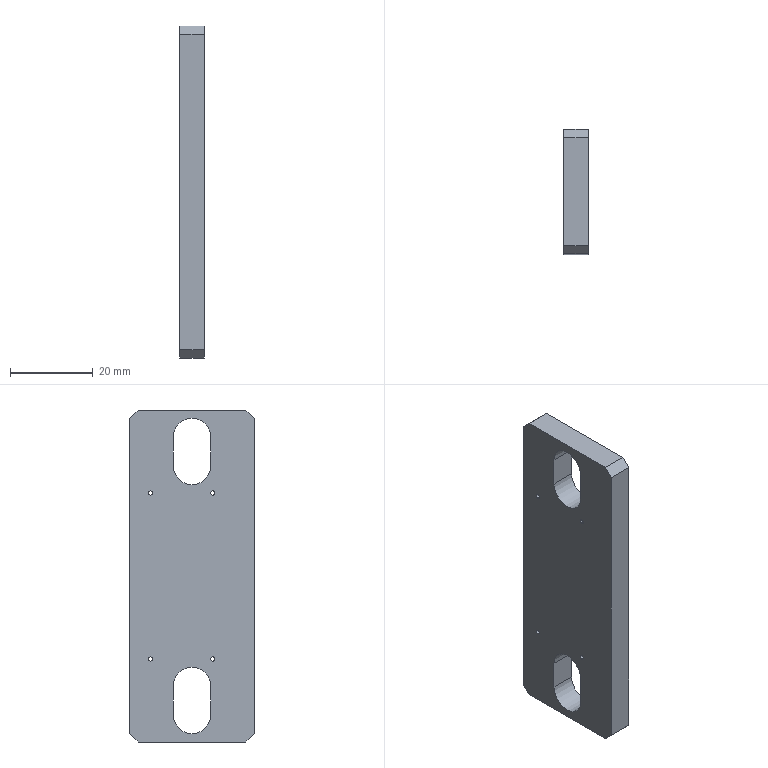Part | NX | features solid 2 | 1 solid | 28 faces | box 6 x 30 x 80 mm | volume 12814 mm3 | cylinder 14 | plane 14 | commonest cylinder face diameters 1 x8 9 x6
STEP:
#1=CARTESIAN_POINT('',(-318.,-642.5,316.));
#2=VERTEX_POINT('',#1);
#3=CARTESIAN_POINT('',(-324.,-642.5,316.));
#4=VERTEX_POINT('',#3);
#5=CARTESIAN_POINT('',(-324.,-642.5,316.));
#6=DIRECTION('',(-1.,0.,0.));
#7=VECTOR('',#6,1000.);
#8=LINE('',#5,#7);
#9=EDGE_CURVE('',#2,#4,#8,.T.);
#10=ORIENTED_EDGE('',*,*,#9,.F.);
#11=CARTESIAN_POINT('',(-318.,-647.,311.5));
#12=VERTEX_POINT('',#11);
#13=CARTESIAN_POINT('',(-318.,-642.5,311.5));
#14=DIRECTION('',(-1.,0.,0.));
#15=DIRECTION('',(0.,0.,1.));
#16=AXIS2_PLACEMENT_3D('',#13,#14,#15);
#17=CIRCLE('',#16,4.5);
#18=EDGE_CURVE('',#12,#2,#17,.T.);
#19=ORIENTED_EDGE('',*,*,#18,.F.);
#20=CARTESIAN_POINT('',(-324.,-647.,311.5));
#21=VERTEX_POINT('',#20);
#22=CARTESIAN_POINT('',(-324.,-647.,311.5));
#23=DIRECTION('',(-1.,0.,0.));
#24=VECTOR('',#23,1000.);
#25=LINE('',#22,#24);
#26=EDGE_CURVE('',#12,#21,#25,.T.);
#27=ORIENTED_EDGE('',*,*,#26,.T.);
#28=CARTESIAN_POINT('',(-324.,-642.5,311.5));
#29=DIRECTION('',(-1.,0.,0.));
#30=DIRECTION('',(0.,0.,1.));
#31=AXIS2_PLACEMENT_3D('',#28,#29,#30);
#32=CIRCLE('',#31,4.5);
#33=EDGE_CURVE('',#21,#4,#32,.T.);
#34=ORIENTED_EDGE('',*,*,#33,.T.);
#35=EDGE_LOOP('',(#10,#19,#27,#34));
#36=FACE_BOUND('',#35,.T.);
#37=CARTESIAN_POINT('',(-324.,-642.5,311.5));
#38=DIRECTION('',(-1.,0.,0.));
#39=DIRECTION('',(0.,0.,1.));
#40=AXIS2_PLACEMENT_3D('',#37,#38,#39);
#41=CYLINDRICAL_SURFACE('',#40,4.5);
#42=ADVANCED_FACE('',(#36),#41,.F.);
#43=CARTESIAN_POINT('',(-318.,-647.,304.5));
#44=VERTEX_POINT('',#43);
#45=CARTESIAN_POINT('',(-324.,-647.,304.5));
#46=VERTEX_POINT('',#45);
#47=CARTESIAN_POINT('',(-324.,-647.,304.5));
#48=DIRECTION('',(-1.,0.,0.));
#49=VECTOR('',#48,1000.);
#50=LINE('',#47,#49);
#51=EDGE_CURVE('',#44,#46,#50,.T.);
#52=ORIENTED_EDGE('',*,*,#51,.T.);
#53=CARTESIAN_POINT('',(-324.,-647.,281.194));
#54=DIRECTION('',(0.,0.,1.));
#55=VECTOR('',#54,1000.);
#56=LINE('',#53,#55);
#57=EDGE_CURVE('',#46,#21,#56,.T.);
#58=ORIENTED_EDGE('',*,*,#57,.T.);
#59=ORIENTED_EDGE('',*,*,#26,.F.);
#60=CARTESIAN_POINT('',(-318.,-647.,281.194));
#61=DIRECTION('',(0.,0.,1.));
#62=VECTOR('',#61,1000.);
#63=LINE('',#60,#62);
#64=EDGE_CURVE('',#44,#12,#63,.T.);
#65=ORIENTED_EDGE('',*,*,#64,.F.);
#66=EDGE_LOOP('',(#52,#58,#59,#65));
#67=FACE_BOUND('',#66,.T.);
#68=CARTESIAN_POINT('',(-324.,-647.,281.194));
#69=DIRECTION('',(0.,-1.,0.));
#70=DIRECTION('',(-1.,0.,0.));
#71=AXIS2_PLACEMENT_3D('',#68,#69,#70);
#72=PLANE('',#71);
#73=ADVANCED_FACE('',(#67),#72,.F.);
#74=CARTESIAN_POINT('',(-318.,-638.,304.5));
#75=VERTEX_POINT('',#74);
#76=CARTESIAN_POINT('',(-324.,-638.,304.5));
#77=VERTEX_POINT('',#76);
#78=CARTESIAN_POINT('',(-324.,-638.,304.5));
#79=DIRECTION('',(-1.,0.,0.));
#80=VECTOR('',#79,1000.);
#81=LINE('',#78,#80);
#82=EDGE_CURVE('',#75,#77,#81,.T.);
#83=ORIENTED_EDGE('',*,*,#82,.T.);
#84=CARTESIAN_POINT('',(-324.,-642.5,304.5));
#85=DIRECTION('',(-1.,0.,0.));
#86=DIRECTION('',(0.,0.,1.));
#87=AXIS2_PLACEMENT_3D('',#84,#85,#86);
#88=CIRCLE('',#87,4.5);
#89=EDGE_CURVE('',#77,#46,#88,.T.);
#90=ORIENTED_EDGE('',*,*,#89,.T.);
#91=ORIENTED_EDGE('',*,*,#51,.F.);
#92=CARTESIAN_POINT('',(-318.,-642.5,304.5));
#93=DIRECTION('',(-1.,0.,0.));
#94=DIRECTION('',(0.,0.,1.));
#95=AXIS2_PLACEMENT_3D('',#92,#93,#94);
#96=CIRCLE('',#95,4.5);
#97=EDGE_CURVE('',#75,#44,#96,.T.);
#98=ORIENTED_EDGE('',*,*,#97,.F.);
#99=EDGE_LOOP('',(#83,#90,#91,#98));
#100=FACE_BOUND('',#99,.T.);
#101=CARTESIAN_POINT('',(-324.,-642.5,304.5));
#102=DIRECTION('',(-1.,0.,0.));
#103=DIRECTION('',(0.,0.,1.));
#104=AXIS2_PLACEMENT_3D('',#101,#102,#103);
#105=CYLINDRICAL_SURFACE('',#104,4.5);
#106=ADVANCED_FACE('',(#100),#105,.F.);
#107=CARTESIAN_POINT('',(-318.,-638.,311.5));
#108=VERTEX_POINT('',#107);
#109=CARTESIAN_POINT('',(-324.,-638.,311.5));
#110=VERTEX_POINT('',#109);
#111=CARTESIAN_POINT('',(-324.,-638.,311.5));
#112=DIRECTION('',(-1.,0.,0.));
#113=VECTOR('',#112,1000.);
#114=LINE('',#111,#113);
#115=EDGE_CURVE('',#108,#110,#114,.T.);
#116=ORIENTED_EDGE('',*,*,#115,.T.);
#117=CARTESIAN_POINT('',(-324.,-638.,281.194));
#118=DIRECTION('',(0.,0.,-1.));
#119=VECTOR('',#118,1000.);
#120=LINE('',#117,#119);
#121=EDGE_CURVE('',#110,#77,#120,.T.);
#122=ORIENTED_EDGE('',*,*,#121,.T.);
#123=ORIENTED_EDGE('',*,*,#82,.F.);
#124=CARTESIAN_POINT('',(-318.,-638.,281.194));
#125=DIRECTION('',(0.,0.,-1.));
#126=VECTOR('',#125,1000.);
#127=LINE('',#124,#126);
#128=EDGE_CURVE('',#108,#75,#127,.T.);
#129=ORIENTED_EDGE('',*,*,#128,.F.);
#130=EDGE_LOOP('',(#116,#122,#123,#129));
#131=FACE_BOUND('',#130,.T.);
#132=CARTESIAN_POINT('',(-324.,-638.,281.194));
#133=DIRECTION('',(0.,1.,0.));
#134=DIRECTION('',(0.,0.,-1.));
#135=AXIS2_PLACEMENT_3D('',#132,#133,#134);
#136=PLANE('',#135);
#137=ADVANCED_FACE('',(#131),#136,.F.);
#138=CARTESIAN_POINT('',(-318.,-642.5,256.));
#139=VERTEX_POINT('',#138);
#140=CARTESIAN_POINT('',(-324.,-642.5,256.));
#141=VERTEX_POINT('',#140);
#142=CARTESIAN_POINT('',(-324.,-642.5,256.));
#143=DIRECTION('',(-1.,0.,0.));
#144=VECTOR('',#143,1000.);
#145=LINE('',#142,#144);
#146=EDGE_CURVE('',#139,#141,#145,.T.);
#147=ORIENTED_EDGE('',*,*,#146,.F.);
#148=CARTESIAN_POINT('',(-318.,-647.,251.5));
#149=VERTEX_POINT('',#148);
#150=CARTESIAN_POINT('',(-318.,-642.5,251.5));
#151=DIRECTION('',(-1.,0.,0.));
#152=DIRECTION('',(0.,0.,1.));
#153=AXIS2_PLACEMENT_3D('',#150,#151,#152);
#154=CIRCLE('',#153,4.5);
#155=EDGE_CURVE('',#149,#139,#154,.T.);
#156=ORIENTED_EDGE('',*,*,#155,.F.);
#157=CARTESIAN_POINT('',(-324.,-647.,251.5));
#158=VERTEX_POINT('',#157);
#159=CARTESIAN_POINT('',(-324.,-647.,251.5));
#160=DIRECTION('',(-1.,0.,0.));
#161=VECTOR('',#160,1000.);
#162=LINE('',#159,#161);
#163=EDGE_CURVE('',#149,#158,#162,.T.);
#164=ORIENTED_EDGE('',*,*,#163,.T.);
#165=CARTESIAN_POINT('',(-324.,-642.5,251.5));
#166=DIRECTION('',(-1.,0.,0.));
#167=DIRECTION('',(0.,0.,1.));
#168=AXIS2_PLACEMENT_3D('',#165,#166,#167);
#169=CIRCLE('',#168,4.5);
#170=EDGE_CURVE('',#158,#141,#169,.T.);
#171=ORIENTED_EDGE('',*,*,#170,.T.);
#172=EDGE_LOOP('',(#147,#156,#164,#171));
#173=FACE_BOUND('',#172,.T.);
#174=CARTESIAN_POINT('',(-324.,-642.5,251.5));
#175=DIRECTION('',(-1.,0.,0.));
#176=DIRECTION('',(0.,0.,1.));
#177=AXIS2_PLACEMENT_3D('',#174,#175,#176);
#178=CYLINDRICAL_SURFACE('',#177,4.5);
#179=ADVANCED_FACE('',(#173),#178,.F.);
#180=CARTESIAN_POINT('',(-318.,-647.,244.5));
#181=VERTEX_POINT('',#180);
#182=CARTESIAN_POINT('',(-324.,-647.,244.5));
#183=VERTEX_POINT('',#182);
#184=CARTESIAN_POINT('',(-324.,-647.,244.5));
#185=DIRECTION('',(-1.,0.,0.));
#186=VECTOR('',#185,1000.);
#187=LINE('',#184,#186);
#188=EDGE_CURVE('',#181,#183,#187,.T.);
#189=ORIENTED_EDGE('',*,*,#188,.T.);
#190=CARTESIAN_POINT('',(-324.,-647.,281.194));
#191=DIRECTION('',(0.,0.,1.));
#192=VECTOR('',#191,1000.);
#193=LINE('',#190,#192);
#194=EDGE_CURVE('',#183,#158,#193,.T.);
#195=ORIENTED_EDGE('',*,*,#194,.T.);
#196=ORIENTED_EDGE('',*,*,#163,.F.);
#197=CARTESIAN_POINT('',(-318.,-647.,281.194));
#198=DIRECTION('',(0.,0.,1.));
#199=VECTOR('',#198,1000.);
#200=LINE('',#197,#199);
#201=EDGE_CURVE('',#181,#149,#200,.T.);
#202=ORIENTED_EDGE('',*,*,#201,.F.);
#203=EDGE_LOOP('',(#189,#195,#196,#202));
#204=FACE_BOUND('',#203,.T.);
#205=CARTESIAN_POINT('',(-324.,-647.,281.194));
#206=DIRECTION('',(0.,-1.,0.));
#207=DIRECTION('',(-1.,0.,0.));
#208=AXIS2_PLACEMENT_3D('',#205,#206,#207);
#209=PLANE('',#208);
#210=ADVANCED_FACE('',(#204),#209,.F.);
#211=CARTESIAN_POINT('',(-318.,-638.,244.5));
#212=VERTEX_POINT('',#211);
#213=CARTESIAN_POINT('',(-324.,-638.,244.5));
#214=VERTEX_POINT('',#213);
#215=CARTESIAN_POINT('',(-324.,-638.,244.5));
#216=DIRECTION('',(-1.,0.,0.));
#217=VECTOR('',#216,1000.);
#218=LINE('',#215,#217);
#219=EDGE_CURVE('',#212,#214,#218,.T.);
#220=ORIENTED_EDGE('',*,*,#219,.T.);
#221=CARTESIAN_POINT('',(-324.,-642.5,244.5));
#222=DIRECTION('',(-1.,0.,0.));
#223=DIRECTION('',(0.,0.,1.));
#224=AXIS2_PLACEMENT_3D('',#221,#222,#223);
#225=CIRCLE('',#224,4.5);
#226=EDGE_CURVE('',#214,#183,#225,.T.);
#227=ORIENTED_EDGE('',*,*,#226,.T.);
#228=ORIENTED_EDGE('',*,*,#188,.F.);
#229=CARTESIAN_POINT('',(-318.,-642.5,244.5));
#230=DIRECTION('',(-1.,0.,0.));
#231=DIRECTION('',(0.,0.,1.));
#232=AXIS2_PLACEMENT_3D('',#229,#230,#231);
#233=CIRCLE('',#232,4.5);
#234=EDGE_CURVE('',#212,#181,#233,.T.);
#235=ORIENTED_EDGE('',*,*,#234,.F.);
#236=EDGE_LOOP('',(#220,#227,#228,#235));
#237=FACE_BOUND('',#236,.T.);
#238=CARTESIAN_POINT('',(-324.,-642.5,244.5));
#239=DIRECTION('',(-1.,0.,0.));
#240=DIRECTION('',(0.,0.,1.));
#241=AXIS2_PLACEMENT_3D('',#238,#239,#240);
#242=CYLINDRICAL_SURFACE('',#241,4.5);
#243=ADVANCED_FACE('',(#237),#242,.F.);
#244=CARTESIAN_POINT('',(-318.,-638.,251.5));
#245=VERTEX_POINT('',#244);
#246=CARTESIAN_POINT('',(-324.,-638.,251.5));
#247=VERTEX_POINT('',#246);
#248=CARTESIAN_POINT('',(-324.,-638.,251.5));
#249=DIRECTION('',(-1.,0.,0.));
#250=VECTOR('',#249,1000.);
#251=LINE('',#248,#250);
#252=EDGE_CURVE('',#245,#247,#251,.T.);
#253=ORIENTED_EDGE('',*,*,#252,.T.);
#254=CARTESIAN_POINT('',(-324.,-638.,281.194));
#255=DIRECTION('',(0.,0.,-1.));
#256=VECTOR('',#255,1000.);
#257=LINE('',#254,#256);
#258=EDGE_CURVE('',#247,#214,#257,.T.);
#259=ORIENTED_EDGE('',*,*,#258,.T.);
#260=ORIENTED_EDGE('',*,*,#219,.F.);
#261=CARTESIAN_POINT('',(-318.,-638.,281.194));
#262=DIRECTION('',(0.,0.,-1.));
#263=VECTOR('',#262,1000.);
#264=LINE('',#261,#263);
#265=EDGE_CURVE('',#245,#212,#264,.T.);
#266=ORIENTED_EDGE('',*,*,#265,.F.);
#267=EDGE_LOOP('',(#253,#259,#260,#266));
#268=FACE_BOUND('',#267,.T.);
#269=CARTESIAN_POINT('',(-324.,-638.,281.194));
#270=DIRECTION('',(0.,1.,0.));
#271=DIRECTION('',(0.,0.,-1.));
#272=AXIS2_PLACEMENT_3D('',#269,#270,#271);
#273=PLANE('',#272);
#274=ADVANCED_FACE('',(#268),#273,.F.);
#275=CARTESIAN_POINT('',(-324.,-647.5,257.5));
#276=VERTEX_POINT('',#275);
#277=CARTESIAN_POINT('',(-318.,-647.5,257.5));
#278=VERTEX_POINT('',#277);
#279=CARTESIAN_POINT('',(-238.35,-647.5,257.5));
#280=DIRECTION('',(-1.,0.,0.));
#281=VECTOR('',#280,1000.);
#282=LINE('',#279,#281);
#283=EDGE_CURVE('',#276,#278,#282,.F.);
#284=ORIENTED_EDGE('',*,*,#283,.T.);
#285=CARTESIAN_POINT('',(-318.,-647.5,258.5));
#286=VERTEX_POINT('',#285);
#287=CARTESIAN_POINT('',(-318.,-647.5,258.));
#288=DIRECTION('',(-1.,0.,0.));
#289=DIRECTION('',(0.,0.,1.));
#290=AXIS2_PLACEMENT_3D('',#287,#288,#289);
#291=CIRCLE('',#290,0.5);
#292=EDGE_CURVE('',#286,#278,#291,.T.);
#293=ORIENTED_EDGE('',*,*,#292,.F.);
#294=CARTESIAN_POINT('',(-324.,-647.5,258.5));
#295=VERTEX_POINT('',#294);
#296=CARTESIAN_POINT('',(-238.35,-647.5,258.5));
#297=DIRECTION('',(-1.,0.,0.));
#298=VECTOR('',#297,1000.);
#299=LINE('',#296,#298);
#300=EDGE_CURVE('',#286,#295,#299,.T.);
#301=ORIENTED_EDGE('',*,*,#300,.T.);
#302=CARTESIAN_POINT('',(-324.,-647.5,258.));
#303=DIRECTION('',(-1.,0.,0.));
#304=DIRECTION('',(0.,0.,-1.));
#305=AXIS2_PLACEMENT_3D('',#302,#303,#304);
#306=CIRCLE('',#305,0.5);
#307=EDGE_CURVE('',#295,#276,#306,.T.);
#308=ORIENTED_EDGE('',*,*,#307,.T.);
#309=EDGE_LOOP('',(#284,#293,#301,#308));
#310=FACE_BOUND('',#309,.T.);
#311=CARTESIAN_POINT('',(-238.35,-647.5,258.));
#312=DIRECTION('',(-1.,0.,0.));
#313=DIRECTION('',(0.,0.,1.));
#314=AXIS2_PLACEMENT_3D('',#311,#312,#313);
#315=CYLINDRICAL_SURFACE('',#314,0.5);
#316=ADVANCED_FACE('',(#310),#315,.F.);
#317=CARTESIAN_POINT('',(-324.,-632.5,257.5));
#318=VERTEX_POINT('',#317);
#319=CARTESIAN_POINT('',(-318.,-632.5,257.5));
#320=VERTEX_POINT('',#319);
#321=CARTESIAN_POINT('',(-238.35,-632.5,257.5));
#322=DIRECTION('',(-1.,0.,0.));
#323=VECTOR('',#322,1000.);
#324=LINE('',#321,#323);
#325=EDGE_CURVE('',#318,#320,#324,.F.);
#326=ORIENTED_EDGE('',*,*,#325,.T.);
#327=CARTESIAN_POINT('',(-318.,-632.5,258.5));
#328=VERTEX_POINT('',#327);
#329=CARTESIAN_POINT('',(-318.,-632.5,258.));
#330=DIRECTION('',(-1.,0.,0.));
#331=DIRECTION('',(0.,0.,1.));
#332=AXIS2_PLACEMENT_3D('',#329,#330,#331);
#333=CIRCLE('',#332,0.5);
#334=EDGE_CURVE('',#328,#320,#333,.T.);
#335=ORIENTED_EDGE('',*,*,#334,.F.);
#336=CARTESIAN_POINT('',(-324.,-632.5,258.5));
#337=VERTEX_POINT('',#336);
#338=CARTESIAN_POINT('',(-238.35,-632.5,258.5));
#339=DIRECTION('',(-1.,0.,0.));
#340=VECTOR('',#339,1000.);
#341=LINE('',#338,#340);
#342=EDGE_CURVE('',#328,#337,#341,.T.);
#343=ORIENTED_EDGE('',*,*,#342,.T.);
#344=CARTESIAN_POINT('',(-324.,-632.5,258.));
#345=DIRECTION('',(-1.,0.,0.));
#346=DIRECTION('',(0.,0.,-1.));
#347=AXIS2_PLACEMENT_3D('',#344,#345,#346);
#348=CIRCLE('',#347,0.5);
#349=EDGE_CURVE('',#337,#318,#348,.T.);
#350=ORIENTED_EDGE('',*,*,#349,.T.);
#351=EDGE_LOOP('',(#326,#335,#343,#350));
#352=FACE_BOUND('',#351,.T.);
#353=CARTESIAN_POINT('',(-238.35,-632.5,258.));
#354=DIRECTION('',(-1.,0.,0.));
#355=DIRECTION('',(0.,0.,1.));
#356=AXIS2_PLACEMENT_3D('',#353,#354,#355);
#357=CYLINDRICAL_SURFACE('',#356,0.5);
#358=ADVANCED_FACE('',(#352),#357,.F.);
#359=CARTESIAN_POINT('',(-318.,-632.5,297.5));
#360=VERTEX_POINT('',#359);
#361=CARTESIAN_POINT('',(-324.,-632.5,297.5));
#362=VERTEX_POINT('',#361);
#363=CARTESIAN_POINT('',(-238.35,-632.5,297.5));
#364=DIRECTION('',(-1.,0.,0.));
#365=VECTOR('',#364,1000.);
#366=LINE('',#363,#365);
#367=EDGE_CURVE('',#360,#362,#366,.T.);
#368=ORIENTED_EDGE('',*,*,#367,.F.);
#369=CARTESIAN_POINT('',(-318.,-632.5,298.5));
#370=VERTEX_POINT('',#369);
#371=CARTESIAN_POINT('',(-318.,-632.5,298.));
#372=DIRECTION('',(-1.,0.,0.));
#373=DIRECTION('',(0.,0.,1.));
#374=AXIS2_PLACEMENT_3D('',#371,#372,#373);
#375=CIRCLE('',#374,0.5);
#376=EDGE_CURVE('',#370,#360,#375,.T.);
#377=ORIENTED_EDGE('',*,*,#376,.F.);
#378=CARTESIAN_POINT('',(-324.,-632.5,298.5));
#379=VERTEX_POINT('',#378);
#380=CARTESIAN_POINT('',(-238.35,-632.5,298.5));
#381=DIRECTION('',(-1.,0.,0.));
#382=VECTOR('',#381,1000.);
#383=LINE('',#380,#382);
#384=EDGE_CURVE('',#379,#370,#383,.F.);
#385=ORIENTED_EDGE('',*,*,#384,.F.);
#386=CARTESIAN_POINT('',(-324.,-632.5,298.));
#387=DIRECTION('',(-1.,0.,0.));
#388=DIRECTION('',(0.,0.,-1.));
#389=AXIS2_PLACEMENT_3D('',#386,#387,#388);
#390=CIRCLE('',#389,0.5);
#391=EDGE_CURVE('',#379,#362,#390,.T.);
#392=ORIENTED_EDGE('',*,*,#391,.T.);
#393=EDGE_LOOP('',(#368,#377,#385,#392));
#394=FACE_BOUND('',#393,.T.);
#395=CARTESIAN_POINT('',(-238.35,-632.5,298.));
#396=DIRECTION('',(-1.,0.,0.));
#397=DIRECTION('',(0.,0.,1.));
#398=AXIS2_PLACEMENT_3D('',#395,#396,#397);
#399=CYLINDRICAL_SURFACE('',#398,0.5);
#400=ADVANCED_FACE('',(#394),#399,.F.);
#401=CARTESIAN_POINT('',(-324.,-647.5,297.5));
#402=VERTEX_POINT('',#401);
#403=CARTESIAN_POINT('',(-318.,-647.5,297.5));
#404=VERTEX_POINT('',#403);
#405=CARTESIAN_POINT('',(-238.35,-647.5,297.5));
#406=DIRECTION('',(-1.,0.,0.));
#407=VECTOR('',#406,1000.);
#408=LINE('',#405,#407);
#409=EDGE_CURVE('',#402,#404,#408,.F.);
#410=ORIENTED_EDGE('',*,*,#409,.T.);
#411=CARTESIAN_POINT('',(-318.,-647.5,298.5));
#412=VERTEX_POINT('',#411);
#413=CARTESIAN_POINT('',(-318.,-647.5,298.));
#414=DIRECTION('',(-1.,0.,0.));
#415=DIRECTION('',(0.,0.,1.));
#416=AXIS2_PLACEMENT_3D('',#413,#414,#415);
#417=CIRCLE('',#416,0.5);
#418=EDGE_CURVE('',#412,#404,#417,.T.);
#419=ORIENTED_EDGE('',*,*,#418,.F.);
#420=CARTESIAN_POINT('',(-324.,-647.5,298.5));
#421=VERTEX_POINT('',#420);
#422=CARTESIAN_POINT('',(-238.35,-647.5,298.5));
#423=DIRECTION('',(-1.,0.,0.));
#424=VECTOR('',#423,1000.);
#425=LINE('',#422,#424);
#426=EDGE_CURVE('',#412,#421,#425,.T.);
#427=ORIENTED_EDGE('',*,*,#426,.T.);
#428=CARTESIAN_POINT('',(-324.,-647.5,298.));
#429=DIRECTION('',(-1.,0.,0.));
#430=DIRECTION('',(0.,0.,-1.));
#431=AXIS2_PLACEMENT_3D('',#428,#429,#430);
#432=CIRCLE('',#431,0.5);
#433=EDGE_CURVE('',#421,#402,#432,.T.);
#434=ORIENTED_EDGE('',*,*,#433,.T.);
#435=EDGE_LOOP('',(#410,#419,#427,#434));
#436=FACE_BOUND('',#435,.T.);
#437=CARTESIAN_POINT('',(-238.35,-647.5,298.));
#438=DIRECTION('',(-1.,0.,0.));
#439=DIRECTION('',(0.,0.,1.));
#440=AXIS2_PLACEMENT_3D('',#437,#438,#439);
#441=CYLINDRICAL_SURFACE('',#440,0.5);
#442=ADVANCED_FACE('',(#436),#441,.F.);
#443=ORIENTED_EDGE('',*,*,#433,.F.);
#444=CARTESIAN_POINT('',(-324.,-647.5,298.));
#445=DIRECTION('',(-1.,0.,0.));
#446=DIRECTION('',(0.,0.,-1.));
#447=AXIS2_PLACEMENT_3D('',#444,#445,#446);
#448=CIRCLE('',#447,0.5);
#449=EDGE_CURVE('',#402,#421,#448,.T.);
#450=ORIENTED_EDGE('',*,*,#449,.F.);
#451=EDGE_LOOP('',(#443,#450));
#452=FACE_BOUND('',#451,.T.);
#453=ORIENTED_EDGE('',*,*,#391,.F.);
#454=CARTESIAN_POINT('',(-324.,-632.5,298.));
#455=DIRECTION('',(-1.,0.,0.));
#456=DIRECTION('',(0.,0.,-1.));
#457=AXIS2_PLACEMENT_3D('',#454,#455,#456);
#458=CIRCLE('',#457,0.5);
#459=EDGE_CURVE('',#362,#379,#458,.T.);
#460=ORIENTED_EDGE('',*,*,#459,.F.);
#461=EDGE_LOOP('',(#453,#460));
#462=FACE_BOUND('',#461,.T.);
#463=ORIENTED_EDGE('',*,*,#349,.F.);
#464=CARTESIAN_POINT('',(-324.,-632.5,258.));
#465=DIRECTION('',(-1.,0.,0.));
#466=DIRECTION('',(0.,0.,-1.));
#467=AXIS2_PLACEMENT_3D('',#464,#465,#466);
#468=CIRCLE('',#467,0.5);
#469=EDGE_CURVE('',#318,#337,#468,.T.);
#470=ORIENTED_EDGE('',*,*,#469,.F.);
#471=EDGE_LOOP('',(#463,#470));
#472=FACE_BOUND('',#471,.T.);
#473=ORIENTED_EDGE('',*,*,#307,.F.);
#474=CARTESIAN_POINT('',(-324.,-647.5,258.));
#475=DIRECTION('',(-1.,0.,0.));
#476=DIRECTION('',(0.,0.,-1.));
#477=AXIS2_PLACEMENT_3D('',#474,#475,#476);
#478=CIRCLE('',#477,0.5);
#479=EDGE_CURVE('',#276,#295,#478,.T.);
#480=ORIENTED_EDGE('',*,*,#479,.F.);
#481=EDGE_LOOP('',(#473,#480));
#482=FACE_BOUND('',#481,.T.);
#483=ORIENTED_EDGE('',*,*,#258,.F.);
#484=CARTESIAN_POINT('',(-324.,-642.5,251.5));
#485=DIRECTION('',(-1.,0.,0.));
#486=DIRECTION('',(0.,0.,1.));
#487=AXIS2_PLACEMENT_3D('',#484,#485,#486);
#488=CIRCLE('',#487,4.5);
#489=EDGE_CURVE('',#141,#247,#488,.T.);
#490=ORIENTED_EDGE('',*,*,#489,.F.);
#491=ORIENTED_EDGE('',*,*,#170,.F.);
#492=ORIENTED_EDGE('',*,*,#194,.F.);
#493=ORIENTED_EDGE('',*,*,#226,.F.);
#494=EDGE_LOOP('',(#483,#490,#491,#492,#493));
#495=FACE_BOUND('',#494,.T.);
#496=ORIENTED_EDGE('',*,*,#121,.F.);
#497=CARTESIAN_POINT('',(-324.,-642.5,311.5));
#498=DIRECTION('',(-1.,0.,0.));
#499=DIRECTION('',(0.,0.,1.));
#500=AXIS2_PLACEMENT_3D('',#497,#498,#499);
#501=CIRCLE('',#500,4.5);
#502=EDGE_CURVE('',#4,#110,#501,.T.);
#503=ORIENTED_EDGE('',*,*,#502,.F.);
#504=ORIENTED_EDGE('',*,*,#33,.F.);
#505=ORIENTED_EDGE('',*,*,#57,.F.);
#506=ORIENTED_EDGE('',*,*,#89,.F.);
#507=EDGE_LOOP('',(#496,#503,#504,#505,#506));
#508=FACE_BOUND('',#507,.T.);
#509=CARTESIAN_POINT('',(-324.,-655.5,238.));
#510=VERTEX_POINT('',#509);
#511=CARTESIAN_POINT('',(-324.,-657.5,240.));
#512=VERTEX_POINT('',#511);
#513=CARTESIAN_POINT('',(-324.,-655.5,238.));
#514=DIRECTION('',(0.,-0.7071,0.7071));
#515=VECTOR('',#514,1000.);
#516=LINE('',#513,#515);
#517=EDGE_CURVE('',#510,#512,#516,.T.);
#518=ORIENTED_EDGE('',*,*,#517,.T.);
#519=CARTESIAN_POINT('',(-324.,-657.5,316.));
#520=VERTEX_POINT('',#519);
#521=CARTESIAN_POINT('',(-324.,-657.5,240.));
#522=DIRECTION('',(0.,0.,1.));
#523=VECTOR('',#522,1000.);
#524=LINE('',#521,#523);
#525=EDGE_CURVE('',#512,#520,#524,.T.);
#526=ORIENTED_EDGE('',*,*,#525,.T.);
#527=CARTESIAN_POINT('',(-324.,-655.5,318.));
#528=VERTEX_POINT('',#527);
#529=CARTESIAN_POINT('',(-324.,-657.5,316.));
#530=DIRECTION('',(0.,0.7071,0.7071));
#531=VECTOR('',#530,1000.);
#532=LINE('',#529,#531);
#533=EDGE_CURVE('',#520,#528,#532,.T.);
#534=ORIENTED_EDGE('',*,*,#533,.T.);
#535=CARTESIAN_POINT('',(-324.,-629.5,318.));
#536=VERTEX_POINT('',#535);
#537=CARTESIAN_POINT('',(-324.,-629.5,318.));
#538=DIRECTION('',(0.,1.,0.));
#539=VECTOR('',#538,1000.);
#540=LINE('',#537,#539);
#541=EDGE_CURVE('',#528,#536,#540,.T.);
#542=ORIENTED_EDGE('',*,*,#541,.T.);
#543=CARTESIAN_POINT('',(-324.,-627.5,316.));
#544=VERTEX_POINT('',#543);
#545=CARTESIAN_POINT('',(-324.,-627.5,316.));
#546=DIRECTION('',(0.,0.7071,-0.7071));
#547=VECTOR('',#546,1000.);
#548=LINE('',#545,#547);
#549=EDGE_CURVE('',#536,#544,#548,.T.);
#550=ORIENTED_EDGE('',*,*,#549,.T.);
#551=CARTESIAN_POINT('',(-324.,-627.5,240.));
#552=VERTEX_POINT('',#551);
#553=CARTESIAN_POINT('',(-324.,-627.5,240.));
#554=DIRECTION('',(0.,0.,-1.));
#555=VECTOR('',#554,1000.);
#556=LINE('',#553,#555);
#557=EDGE_CURVE('',#544,#552,#556,.T.);
#558=ORIENTED_EDGE('',*,*,#557,.T.);
#559=CARTESIAN_POINT('',(-324.,-629.5,238.));
#560=VERTEX_POINT('',#559);
#561=CARTESIAN_POINT('',(-324.,-629.5,238.));
#562=DIRECTION('',(0.,-0.7071,-0.7071));
#563=VECTOR('',#562,1000.);
#564=LINE('',#561,#563);
#565=EDGE_CURVE('',#552,#560,#564,.T.);
#566=ORIENTED_EDGE('',*,*,#565,.T.);
#567=CARTESIAN_POINT('',(-324.,-629.5,238.));
#568=DIRECTION('',(0.,-1.,0.));
#569=VECTOR('',#568,1000.);
#570=LINE('',#567,#569);
#571=EDGE_CURVE('',#560,#510,#570,.T.);
#572=ORIENTED_EDGE('',*,*,#571,.T.);
#573=EDGE_LOOP('',(#518,#526,#534,#542,#550,#558,#566,#572));
#574=FACE_BOUND('',#573,.T.);
#575=CARTESIAN_POINT('',(-324.,-642.5,281.194));
#576=DIRECTION('',(-1.,0.,0.));
#577=DIRECTION('',(0.,1.,0.));
#578=AXIS2_PLACEMENT_3D('',#575,#576,#577);
#579=PLANE('',#578);
#580=ADVANCED_FACE('',(#452,#462,#472,#482,#495,#508,#574),#579,.T.);
#581=ORIENTED_EDGE('',*,*,#418,.T.);
#582=CARTESIAN_POINT('',(-318.,-647.5,298.));
#583=DIRECTION('',(-1.,0.,0.));
#584=DIRECTION('',(0.,0.,1.));
#585=AXIS2_PLACEMENT_3D('',#582,#583,#584);
#586=CIRCLE('',#585,0.5);
#587=EDGE_CURVE('',#404,#412,#586,.T.);
#588=ORIENTED_EDGE('',*,*,#587,.T.);
#589=EDGE_LOOP('',(#581,#588));
#590=FACE_BOUND('',#589,.T.);
#591=ORIENTED_EDGE('',*,*,#376,.T.);
#592=CARTESIAN_POINT('',(-318.,-632.5,298.));
#593=DIRECTION('',(-1.,0.,0.));
#594=DIRECTION('',(0.,0.,1.));
#595=AXIS2_PLACEMENT_3D('',#592,#593,#594);
#596=CIRCLE('',#595,0.5);
#597=EDGE_CURVE('',#360,#370,#596,.T.);
#598=ORIENTED_EDGE('',*,*,#597,.T.);
#599=EDGE_LOOP('',(#591,#598));
#600=FACE_BOUND('',#599,.T.);
#601=ORIENTED_EDGE('',*,*,#334,.T.);
#602=CARTESIAN_POINT('',(-318.,-632.5,258.));
#603=DIRECTION('',(-1.,0.,0.));
#604=DIRECTION('',(0.,0.,1.));
#605=AXIS2_PLACEMENT_3D('',#602,#603,#604);
#606=CIRCLE('',#605,0.5);
#607=EDGE_CURVE('',#320,#328,#606,.T.);
#608=ORIENTED_EDGE('',*,*,#607,.T.);
#609=EDGE_LOOP('',(#601,#608));
#610=FACE_BOUND('',#609,.T.);
#611=ORIENTED_EDGE('',*,*,#292,.T.);
#612=CARTESIAN_POINT('',(-318.,-647.5,258.));
#613=DIRECTION('',(-1.,0.,0.));
#614=DIRECTION('',(0.,0.,1.));
#615=AXIS2_PLACEMENT_3D('',#612,#613,#614);
#616=CIRCLE('',#615,0.5);
#617=EDGE_CURVE('',#278,#286,#616,.T.);
#618=ORIENTED_EDGE('',*,*,#617,.T.);
#619=EDGE_LOOP('',(#611,#618));
#620=FACE_BOUND('',#619,.T.);
#621=ORIENTED_EDGE('',*,*,#155,.T.);
#622=CARTESIAN_POINT('',(-318.,-642.5,251.5));
#623=DIRECTION('',(-1.,0.,0.));
#624=DIRECTION('',(0.,0.,1.));
#625=AXIS2_PLACEMENT_3D('',#622,#623,#624);
#626=CIRCLE('',#625,4.5);
#627=EDGE_CURVE('',#139,#245,#626,.T.);
#628=ORIENTED_EDGE('',*,*,#627,.T.);
#629=ORIENTED_EDGE('',*,*,#265,.T.);
#630=ORIENTED_EDGE('',*,*,#234,.T.);
#631=ORIENTED_EDGE('',*,*,#201,.T.);
#632=EDGE_LOOP('',(#621,#628,#629,#630,#631));
#633=FACE_BOUND('',#632,.T.);
#634=ORIENTED_EDGE('',*,*,#18,.T.);
#635=CARTESIAN_POINT('',(-318.,-642.5,311.5));
#636=DIRECTION('',(-1.,0.,0.));
#637=DIRECTION('',(0.,0.,1.));
#638=AXIS2_PLACEMENT_3D('',#635,#636,#637);
#639=CIRCLE('',#638,4.5);
#640=EDGE_CURVE('',#2,#108,#639,.T.);
#641=ORIENTED_EDGE('',*,*,#640,.T.);
#642=ORIENTED_EDGE('',*,*,#128,.T.);
#643=ORIENTED_EDGE('',*,*,#97,.T.);
#644=ORIENTED_EDGE('',*,*,#64,.T.);
#645=EDGE_LOOP('',(#634,#641,#642,#643,#644));
#646=FACE_BOUND('',#645,.T.);
#647=CARTESIAN_POINT('',(-318.,-655.5,238.));
#648=VERTEX_POINT('',#647);
#649=CARTESIAN_POINT('',(-318.,-657.5,240.));
#650=VERTEX_POINT('',#649);
#651=CARTESIAN_POINT('',(-318.,-655.5,238.));
#652=DIRECTION('',(0.,-0.7071,0.7071));
#653=VECTOR('',#652,1000.);
#654=LINE('',#651,#653);
#655=EDGE_CURVE('',#648,#650,#654,.T.);
#656=ORIENTED_EDGE('',*,*,#655,.F.);
#657=CARTESIAN_POINT('',(-318.,-629.5,238.));
#658=VERTEX_POINT('',#657);
#659=CARTESIAN_POINT('',(-318.,-629.5,238.));
#660=DIRECTION('',(0.,-1.,0.));
#661=VECTOR('',#660,1000.);
#662=LINE('',#659,#661);
#663=EDGE_CURVE('',#658,#648,#662,.T.);
#664=ORIENTED_EDGE('',*,*,#663,.F.);
#665=CARTESIAN_POINT('',(-318.,-627.5,240.));
#666=VERTEX_POINT('',#665);
#667=CARTESIAN_POINT('',(-318.,-629.5,238.));
#668=DIRECTION('',(0.,-0.7071,-0.7071));
#669=VECTOR('',#668,1000.);
#670=LINE('',#667,#669);
#671=EDGE_CURVE('',#666,#658,#670,.T.);
#672=ORIENTED_EDGE('',*,*,#671,.F.);
#673=CARTESIAN_POINT('',(-318.,-627.5,316.));
#674=VERTEX_POINT('',#673);
#675=CARTESIAN_POINT('',(-318.,-627.5,240.));
#676=DIRECTION('',(0.,0.,-1.));
#677=VECTOR('',#676,1000.);
#678=LINE('',#675,#677);
#679=EDGE_CURVE('',#674,#666,#678,.T.);
#680=ORIENTED_EDGE('',*,*,#679,.F.);
#681=CARTESIAN_POINT('',(-318.,-629.5,318.));
#682=VERTEX_POINT('',#681);
#683=CARTESIAN_POINT('',(-318.,-627.5,316.));
#684=DIRECTION('',(0.,0.7071,-0.7071));
#685=VECTOR('',#684,1000.);
#686=LINE('',#683,#685);
#687=EDGE_CURVE('',#682,#674,#686,.T.);
#688=ORIENTED_EDGE('',*,*,#687,.F.);
#689=CARTESIAN_POINT('',(-318.,-655.5,318.));
#690=VERTEX_POINT('',#689);
#691=CARTESIAN_POINT('',(-318.,-629.5,318.));
#692=DIRECTION('',(0.,1.,0.));
#693=VECTOR('',#692,1000.);
#694=LINE('',#691,#693);
#695=EDGE_CURVE('',#690,#682,#694,.T.);
#696=ORIENTED_EDGE('',*,*,#695,.F.);
#697=CARTESIAN_POINT('',(-318.,-657.5,316.));
#698=VERTEX_POINT('',#697);
#699=CARTESIAN_POINT('',(-318.,-657.5,316.));
#700=DIRECTION('',(0.,0.7071,0.7071));
#701=VECTOR('',#700,1000.);
#702=LINE('',#699,#701);
#703=EDGE_CURVE('',#698,#690,#702,.T.);
#704=ORIENTED_EDGE('',*,*,#703,.F.);
#705=CARTESIAN_POINT('',(-318.,-657.5,240.));
#706=DIRECTION('',(0.,0.,1.));
#707=VECTOR('',#706,1000.);
#708=LINE('',#705,#707);
#709=EDGE_CURVE('',#650,#698,#708,.T.);
#710=ORIENTED_EDGE('',*,*,#709,.F.);
#711=EDGE_LOOP('',(#656,#664,#672,#680,#688,#696,#704,#710));
#712=FACE_BOUND('',#711,.T.);
#713=CARTESIAN_POINT('',(-318.,-642.5,281.194));
#714=DIRECTION('',(-1.,0.,0.));
#715=DIRECTION('',(0.,1.,0.));
#716=AXIS2_PLACEMENT_3D('',#713,#714,#715);
#717=PLANE('',#716);
#718=ADVANCED_FACE('',(#590,#600,#610,#620,#633,#646,#712),#717,.F.);
#719=ORIENTED_EDGE('',*,*,#571,.F.);
#720=CARTESIAN_POINT('',(-318.,-629.5,238.));
#721=DIRECTION('',(-1.,0.,0.));
#722=VECTOR('',#721,1000.);
#723=LINE('',#720,#722);
#724=EDGE_CURVE('',#658,#560,#723,.T.);
#725=ORIENTED_EDGE('',*,*,#724,.F.);
#726=ORIENTED_EDGE('',*,*,#663,.T.);
#727=CARTESIAN_POINT('',(-318.,-655.5,238.));
#728=DIRECTION('',(-1.,0.,0.));
#729=VECTOR('',#728,1000.);
#730=LINE('',#727,#729);
#731=EDGE_CURVE('',#648,#510,#730,.T.);
#732=ORIENTED_EDGE('',*,*,#731,.T.);
#733=EDGE_LOOP('',(#719,#725,#726,#732));
#734=FACE_BOUND('',#733,.T.);
#735=CARTESIAN_POINT('',(-318.,-629.5,238.));
#736=DIRECTION('',(0.,0.,-1.));
#737=DIRECTION('',(-1.,0.,0.));
#738=AXIS2_PLACEMENT_3D('',#735,#736,#737);
#739=PLANE('',#738);
#740=ADVANCED_FACE('',(#734),#739,.T.);
#741=ORIENTED_EDGE('',*,*,#565,.F.);
#742=CARTESIAN_POINT('',(-318.,-627.5,240.));
#743=DIRECTION('',(-1.,0.,0.));
#744=VECTOR('',#743,1000.);
#745=LINE('',#742,#744);
#746=EDGE_CURVE('',#666,#552,#745,.T.);
#747=ORIENTED_EDGE('',*,*,#746,.F.);
#748=ORIENTED_EDGE('',*,*,#671,.T.);
#749=ORIENTED_EDGE('',*,*,#724,.T.);
#750=EDGE_LOOP('',(#741,#747,#748,#749));
#751=FACE_BOUND('',#750,.T.);
#752=CARTESIAN_POINT('',(-318.,-629.5,238.));
#753=DIRECTION('',(0.,0.7071,-0.7071));
#754=DIRECTION('',(-1.,0.,0.));
#755=AXIS2_PLACEMENT_3D('',#752,#753,#754);
#756=PLANE('',#755);
#757=ADVANCED_FACE('',(#751),#756,.T.);
#758=ORIENTED_EDGE('',*,*,#557,.F.);
#759=CARTESIAN_POINT('',(-318.,-627.5,316.));
#760=DIRECTION('',(-1.,0.,0.));
#761=VECTOR('',#760,1000.);
#762=LINE('',#759,#761);
#763=EDGE_CURVE('',#674,#544,#762,.T.);
#764=ORIENTED_EDGE('',*,*,#763,.F.);
#765=ORIENTED_EDGE('',*,*,#679,.T.);
#766=ORIENTED_EDGE('',*,*,#746,.T.);
#767=EDGE_LOOP('',(#758,#764,#765,#766));
#768=FACE_BOUND('',#767,.T.);
#769=CARTESIAN_POINT('',(-318.,-627.5,240.));
#770=DIRECTION('',(0.,1.,0.));
#771=DIRECTION('',(0.,0.,-1.));
#772=AXIS2_PLACEMENT_3D('',#769,#770,#771);
#773=PLANE('',#772);
#774=ADVANCED_FACE('',(#768),#773,.T.);
#775=ORIENTED_EDGE('',*,*,#549,.F.);
#776=CARTESIAN_POINT('',(-318.,-629.5,318.));
#777=DIRECTION('',(-1.,0.,0.));
#778=VECTOR('',#777,1000.);
#779=LINE('',#776,#778);
#780=EDGE_CURVE('',#682,#536,#779,.T.);
#781=ORIENTED_EDGE('',*,*,#780,.F.);
#782=ORIENTED_EDGE('',*,*,#687,.T.);
#783=ORIENTED_EDGE('',*,*,#763,.T.);
#784=EDGE_LOOP('',(#775,#781,#782,#783));
#785=FACE_BOUND('',#784,.T.);
#786=CARTESIAN_POINT('',(-318.,-627.5,316.));
#787=DIRECTION('',(0.,0.7071,0.7071));
#788=DIRECTION('',(1.,0.,0.));
#789=AXIS2_PLACEMENT_3D('',#786,#787,#788);
#790=PLANE('',#789);
#791=ADVANCED_FACE('',(#785),#790,.T.);
#792=ORIENTED_EDGE('',*,*,#541,.F.);
#793=CARTESIAN_POINT('',(-318.,-655.5,318.));
#794=DIRECTION('',(-1.,0.,0.));
#795=VECTOR('',#794,1000.);
#796=LINE('',#793,#795);
#797=EDGE_CURVE('',#690,#528,#796,.T.);
#798=ORIENTED_EDGE('',*,*,#797,.F.);
#799=ORIENTED_EDGE('',*,*,#695,.T.);
#800=ORIENTED_EDGE('',*,*,#780,.T.);
#801=EDGE_LOOP('',(#792,#798,#799,#800));
#802=FACE_BOUND('',#801,.T.);
#803=CARTESIAN_POINT('',(-318.,-629.5,318.));
#804=DIRECTION('',(0.,0.,1.));
#805=DIRECTION('',(1.,0.,0.));
#806=AXIS2_PLACEMENT_3D('',#803,#804,#805);
#807=PLANE('',#806);
#808=ADVANCED_FACE('',(#802),#807,.T.);
#809=ORIENTED_EDGE('',*,*,#533,.F.);
#810=CARTESIAN_POINT('',(-318.,-657.5,316.));
#811=DIRECTION('',(-1.,0.,0.));
#812=VECTOR('',#811,1000.);
#813=LINE('',#810,#812);
#814=EDGE_CURVE('',#698,#520,#813,.T.);
#815=ORIENTED_EDGE('',*,*,#814,.F.);
#816=ORIENTED_EDGE('',*,*,#703,.T.);
#817=ORIENTED_EDGE('',*,*,#797,.T.);
#818=EDGE_LOOP('',(#809,#815,#816,#817));
#819=FACE_BOUND('',#818,.T.);
#820=CARTESIAN_POINT('',(-318.,-657.5,316.));
#821=DIRECTION('',(0.,-0.7071,0.7071));
#822=DIRECTION('',(-1.,0.,0.));
#823=AXIS2_PLACEMENT_3D('',#820,#821,#822);
#824=PLANE('',#823);
#825=ADVANCED_FACE('',(#819),#824,.T.);
#826=ORIENTED_EDGE('',*,*,#525,.F.);
#827=CARTESIAN_POINT('',(-318.,-657.5,240.));
#828=DIRECTION('',(-1.,0.,0.));
#829=VECTOR('',#828,1000.);
#830=LINE('',#827,#829);
#831=EDGE_CURVE('',#650,#512,#830,.T.);
#832=ORIENTED_EDGE('',*,*,#831,.F.);
#833=ORIENTED_EDGE('',*,*,#709,.T.);
#834=ORIENTED_EDGE('',*,*,#814,.T.);
#835=EDGE_LOOP('',(#826,#832,#833,#834));
#836=FACE_BOUND('',#835,.T.);
#837=CARTESIAN_POINT('',(-318.,-657.5,240.));
#838=DIRECTION('',(0.,-1.,0.));
#839=DIRECTION('',(-1.,0.,0.));
#840=AXIS2_PLACEMENT_3D('',#837,#838,#839);
#841=PLANE('',#840);
#842=ADVANCED_FACE('',(#836),#841,.T.);
#843=ORIENTED_EDGE('',*,*,#517,.F.);
#844=ORIENTED_EDGE('',*,*,#731,.F.);
#845=ORIENTED_EDGE('',*,*,#655,.T.);
#846=ORIENTED_EDGE('',*,*,#831,.T.);
#847=EDGE_LOOP('',(#843,#844,#845,#846));
#848=FACE_BOUND('',#847,.T.);
#849=CARTESIAN_POINT('',(-318.,-655.5,238.));
#850=DIRECTION('',(0.,-0.7071,-0.7071));
#851=DIRECTION('',(0.,-0.7071,0.7071));
#852=AXIS2_PLACEMENT_3D('',#849,#850,#851);
#853=PLANE('',#852);
#854=ADVANCED_FACE('',(#848),#853,.T.);
#855=ORIENTED_EDGE('',*,*,#587,.F.);
#856=ORIENTED_EDGE('',*,*,#409,.F.);
#857=ORIENTED_EDGE('',*,*,#449,.T.);
#858=ORIENTED_EDGE('',*,*,#426,.F.);
#859=EDGE_LOOP('',(#855,#856,#857,#858));
#860=FACE_BOUND('',#859,.T.);
#861=CARTESIAN_POINT('',(-238.35,-647.5,298.));
#862=DIRECTION('',(-1.,0.,0.));
#863=DIRECTION('',(0.,0.,1.));
#864=AXIS2_PLACEMENT_3D('',#861,#862,#863);
#865=CYLINDRICAL_SURFACE('',#864,0.5);
#866=ADVANCED_FACE('',(#860),#865,.F.);
#867=ORIENTED_EDGE('',*,*,#597,.F.);
#868=ORIENTED_EDGE('',*,*,#367,.T.);
#869=ORIENTED_EDGE('',*,*,#459,.T.);
#870=ORIENTED_EDGE('',*,*,#384,.T.);
#871=EDGE_LOOP('',(#867,#868,#869,#870));
#872=FACE_BOUND('',#871,.T.);
#873=CARTESIAN_POINT('',(-238.35,-632.5,298.));
#874=DIRECTION('',(-1.,0.,0.));
#875=DIRECTION('',(0.,0.,1.));
#876=AXIS2_PLACEMENT_3D('',#873,#874,#875);
#877=CYLINDRICAL_SURFACE('',#876,0.5);
#878=ADVANCED_FACE('',(#872),#877,.F.);
#879=ORIENTED_EDGE('',*,*,#607,.F.);
#880=ORIENTED_EDGE('',*,*,#325,.F.);
#881=ORIENTED_EDGE('',*,*,#469,.T.);
#882=ORIENTED_EDGE('',*,*,#342,.F.);
#883=EDGE_LOOP('',(#879,#880,#881,#882));
#884=FACE_BOUND('',#883,.T.);
#885=CARTESIAN_POINT('',(-238.35,-632.5,258.));
#886=DIRECTION('',(-1.,0.,0.));
#887=DIRECTION('',(0.,0.,1.));
#888=AXIS2_PLACEMENT_3D('',#885,#886,#887);
#889=CYLINDRICAL_SURFACE('',#888,0.5);
#890=ADVANCED_FACE('',(#884),#889,.F.);
#891=ORIENTED_EDGE('',*,*,#617,.F.);
#892=ORIENTED_EDGE('',*,*,#283,.F.);
#893=ORIENTED_EDGE('',*,*,#479,.T.);
#894=ORIENTED_EDGE('',*,*,#300,.F.);
#895=EDGE_LOOP('',(#891,#892,#893,#894));
#896=FACE_BOUND('',#895,.T.);
#897=CARTESIAN_POINT('',(-238.35,-647.5,258.));
#898=DIRECTION('',(-1.,0.,0.));
#899=DIRECTION('',(0.,0.,1.));
#900=AXIS2_PLACEMENT_3D('',#897,#898,#899);
#901=CYLINDRICAL_SURFACE('',#900,0.5);
#902=ADVANCED_FACE('',(#896),#901,.F.);
#903=ORIENTED_EDGE('',*,*,#627,.F.);
#904=ORIENTED_EDGE('',*,*,#146,.T.);
#905=ORIENTED_EDGE('',*,*,#489,.T.);
#906=ORIENTED_EDGE('',*,*,#252,.F.);
#907=EDGE_LOOP('',(#903,#904,#905,#906));
#908=FACE_BOUND('',#907,.T.);
#909=CARTESIAN_POINT('',(-324.,-642.5,251.5));
#910=DIRECTION('',(-1.,0.,0.));
#911=DIRECTION('',(0.,0.,1.));
#912=AXIS2_PLACEMENT_3D('',#909,#910,#911);
#913=CYLINDRICAL_SURFACE('',#912,4.5);
#914=ADVANCED_FACE('',(#908),#913,.F.);
#915=ORIENTED_EDGE('',*,*,#640,.F.);
#916=ORIENTED_EDGE('',*,*,#9,.T.);
#917=ORIENTED_EDGE('',*,*,#502,.T.);
#918=ORIENTED_EDGE('',*,*,#115,.F.);
#919=EDGE_LOOP('',(#915,#916,#917,#918));
#920=FACE_BOUND('',#919,.T.);
#921=CARTESIAN_POINT('',(-324.,-642.5,311.5));
#922=DIRECTION('',(-1.,0.,0.));
#923=DIRECTION('',(0.,0.,1.));
#924=AXIS2_PLACEMENT_3D('',#921,#922,#923);
#925=CYLINDRICAL_SURFACE('',#924,4.5);
#926=ADVANCED_FACE('',(#920),#925,.F.);
#927=CLOSED_SHELL('',(#42,#73,#106,#137,#179,#210,#243,#274,#316,#358,#400,#442,#580,#718,#740,#757,#774,#791,#808,#825,#842,#854,#866,#878,#890,#902,#914,#926));
#928=MANIFOLD_SOLID_BREP('',#927);
#929=(LENGTH_UNIT()NAMED_UNIT(*)SI_UNIT(.MILLI.,.METRE.));
#930=UNCERTAINTY_MEASURE_WITH_UNIT(LENGTH_MEASURE(0.00001),#929,'','');
#931=(NAMED_UNIT(*)PLANE_ANGLE_UNIT()SI_UNIT($,.RADIAN.));
#932=(NAMED_UNIT(*)SI_UNIT($,.STERADIAN.)SOLID_ANGLE_UNIT());
#933=(GEOMETRIC_REPRESENTATION_CONTEXT(3)GLOBAL_UNCERTAINTY_ASSIGNED_CONTEXT((#930))GLOBAL_UNIT_ASSIGNED_CONTEXT((#929,#931,#932))REPRESENTATION_CONTEXT('',''));
#934=ADVANCED_BREP_SHAPE_REPRESENTATION('',(#928),#933);